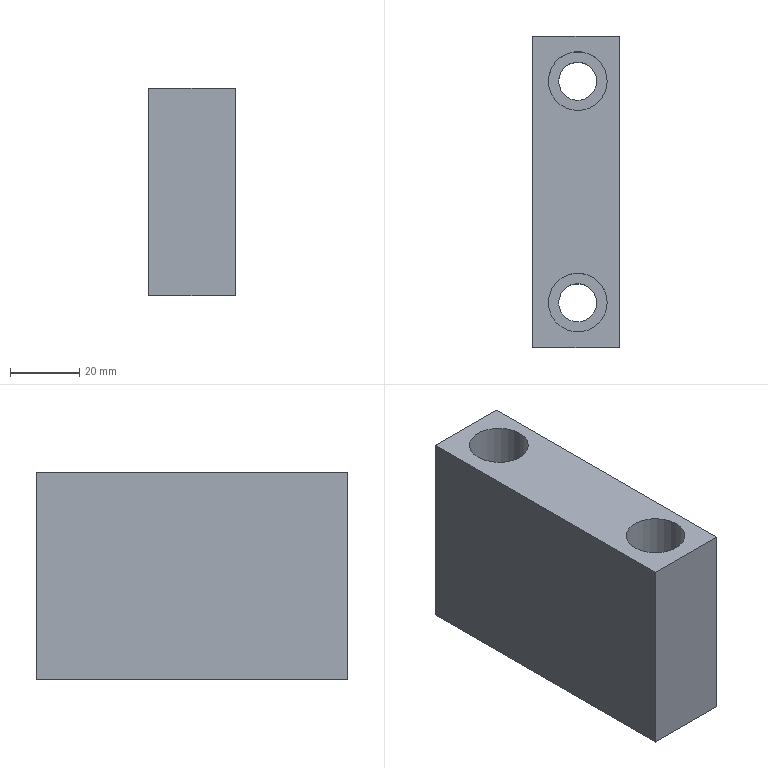Part | STEP file | PN_0005_id1498_x_t | 1 solid | 12 faces | box 25 x 90 x 60 mm | volume 115679 mm3 | plane 8 | cylinder 4 | commonest cylinder face diameters 11 x2 17 x2
STEP:
#1=CARTESIAN_POINT('',(-216.5,194.,155.));
#2=VERTEX_POINT('',#1);
#3=CARTESIAN_POINT('',(-222.,194.,155.));
#4=DIRECTION('',(0.,0.,-1.));
#5=DIRECTION('',(1.,0.,0.));
#6=AXIS2_PLACEMENT_3D('',#3,#4,#5);
#7=CIRCLE('',#6,5.5);
#8=EDGE_CURVE('',#2,#2,#7,.T.);
#9=ORIENTED_EDGE('',*,*,#8,.F.);
#10=EDGE_LOOP('',(#9));
#11=FACE_BOUND('',#10,.T.);
#12=CARTESIAN_POINT('',(-216.5,130.,155.));
#13=VERTEX_POINT('',#12);
#14=CARTESIAN_POINT('',(-222.,130.,155.));
#15=DIRECTION('',(0.,0.,1.));
#16=DIRECTION('',(1.,0.,0.));
#17=AXIS2_PLACEMENT_3D('',#14,#15,#16);
#18=CIRCLE('',#17,5.5);
#19=EDGE_CURVE('',#13,#13,#18,.T.);
#20=ORIENTED_EDGE('',*,*,#19,.T.);
#21=EDGE_LOOP('',(#20));
#22=FACE_BOUND('',#21,.T.);
#23=CARTESIAN_POINT('',(-210.,207.,155.));
#24=VERTEX_POINT('',#23);
#25=CARTESIAN_POINT('',(-235.,207.,155.));
#26=VERTEX_POINT('',#25);
#27=CARTESIAN_POINT('',(-190.,207.,155.));
#28=DIRECTION('',(-1.,0.,0.));
#29=VECTOR('',#28,1.);
#30=LINE('',#27,#29);
#31=EDGE_CURVE('',#24,#26,#30,.T.);
#32=ORIENTED_EDGE('',*,*,#31,.F.);
#33=CARTESIAN_POINT('',(-210.,117.,155.));
#34=VERTEX_POINT('',#33);
#35=CARTESIAN_POINT('',(-210.,-7.4,155.));
#36=DIRECTION('',(0.,-1.,0.));
#37=VECTOR('',#36,1.);
#38=LINE('',#35,#37);
#39=EDGE_CURVE('',#24,#34,#38,.T.);
#40=ORIENTED_EDGE('',*,*,#39,.T.);
#41=CARTESIAN_POINT('',(-235.,117.,155.));
#42=VERTEX_POINT('',#41);
#43=CARTESIAN_POINT('',(-190.,117.,155.));
#44=DIRECTION('',(1.,0.,0.));
#45=VECTOR('',#44,1.);
#46=LINE('',#43,#45);
#47=EDGE_CURVE('',#42,#34,#46,.T.);
#48=ORIENTED_EDGE('',*,*,#47,.F.);
#49=CARTESIAN_POINT('',(-235.,94.6,155.));
#50=DIRECTION('',(0.,-1.,0.));
#51=VECTOR('',#50,1.);
#52=LINE('',#49,#51);
#53=EDGE_CURVE('',#26,#42,#52,.T.);
#54=ORIENTED_EDGE('',*,*,#53,.F.);
#55=EDGE_LOOP('',(#32,#40,#48,#54));
#56=FACE_BOUND('',#55,.T.);
#57=CARTESIAN_POINT('',(223.5,101.,155.));
#58=DIRECTION('',(0.,0.,-1.));
#59=DIRECTION('',(1.,0.,0.));
#60=AXIS2_PLACEMENT_3D('',#57,#58,#59);
#61=PLANE('',#60);
#62=ADVANCED_FACE('',(#11,#22,#56),#61,.T.);
#63=CARTESIAN_POINT('',(-210.,117.,215.));
#64=VERTEX_POINT('',#63);
#65=CARTESIAN_POINT('',(-210.,117.,155.));
#66=DIRECTION('',(0.,0.,-1.));
#67=VECTOR('',#66,1.);
#68=LINE('',#65,#67);
#69=EDGE_CURVE('',#64,#34,#68,.T.);
#70=ORIENTED_EDGE('',*,*,#69,.F.);
#71=CARTESIAN_POINT('',(-235.,117.,215.));
#72=VERTEX_POINT('',#71);
#73=CARTESIAN_POINT('',(-190.,117.,215.));
#74=DIRECTION('',(-1.,0.,0.));
#75=VECTOR('',#74,1.);
#76=LINE('',#73,#75);
#77=EDGE_CURVE('',#64,#72,#76,.T.);
#78=ORIENTED_EDGE('',*,*,#77,.T.);
#79=CARTESIAN_POINT('',(-235.,117.,155.));
#80=DIRECTION('',(0.,0.,-1.));
#81=VECTOR('',#80,1.);
#82=LINE('',#79,#81);
#83=EDGE_CURVE('',#72,#42,#82,.T.);
#84=ORIENTED_EDGE('',*,*,#83,.T.);
#85=ORIENTED_EDGE('',*,*,#47,.T.);
#86=EDGE_LOOP('',(#70,#78,#84,#85));
#87=FACE_OUTER_BOUND('',#86,.T.);
#88=CARTESIAN_POINT('',(-190.,117.,155.));
#89=DIRECTION('',(0.,-1.,0.));
#90=DIRECTION('',(0.,0.,-1.));
#91=AXIS2_PLACEMENT_3D('',#88,#89,#90);
#92=PLANE('',#91);
#93=ADVANCED_FACE('',(#87),#92,.T.);
#94=CARTESIAN_POINT('',(-210.,207.,215.));
#95=VERTEX_POINT('',#94);
#96=CARTESIAN_POINT('',(-210.,207.,155.));
#97=DIRECTION('',(0.,0.,1.));
#98=VECTOR('',#97,1.);
#99=LINE('',#96,#98);
#100=EDGE_CURVE('',#24,#95,#99,.T.);
#101=ORIENTED_EDGE('',*,*,#100,.F.);
#102=ORIENTED_EDGE('',*,*,#31,.T.);
#103=CARTESIAN_POINT('',(-235.,207.,215.));
#104=VERTEX_POINT('',#103);
#105=CARTESIAN_POINT('',(-235.,207.,138.004));
#106=DIRECTION('',(0.,0.,-1.));
#107=VECTOR('',#106,1.);
#108=LINE('',#105,#107);
#109=EDGE_CURVE('',#104,#26,#108,.T.);
#110=ORIENTED_EDGE('',*,*,#109,.F.);
#111=CARTESIAN_POINT('',(-190.,207.,215.));
#112=DIRECTION('',(1.,0.,0.));
#113=VECTOR('',#112,1.);
#114=LINE('',#111,#113);
#115=EDGE_CURVE('',#104,#95,#114,.T.);
#116=ORIENTED_EDGE('',*,*,#115,.T.);
#117=EDGE_LOOP('',(#101,#102,#110,#116));
#118=FACE_OUTER_BOUND('',#117,.T.);
#119=CARTESIAN_POINT('',(-190.,207.,155.));
#120=DIRECTION('',(0.,1.,0.));
#121=DIRECTION('',(0.,0.,1.));
#122=AXIS2_PLACEMENT_3D('',#119,#120,#121);
#123=PLANE('',#122);
#124=ADVANCED_FACE('',(#118),#123,.T.);
#125=CARTESIAN_POINT('',(-230.5,194.,215.));
#126=VERTEX_POINT('',#125);
#127=CARTESIAN_POINT('',(-222.,194.,215.));
#128=DIRECTION('',(0.,0.,1.));
#129=DIRECTION('',(-1.,0.,0.));
#130=AXIS2_PLACEMENT_3D('',#127,#128,#129);
#131=CIRCLE('',#130,8.5);
#132=EDGE_CURVE('',#126,#126,#131,.T.);
#133=ORIENTED_EDGE('',*,*,#132,.F.);
#134=EDGE_LOOP('',(#133));
#135=FACE_BOUND('',#134,.T.);
#136=CARTESIAN_POINT('',(-230.5,130.,215.));
#137=VERTEX_POINT('',#136);
#138=CARTESIAN_POINT('',(-222.,130.,215.));
#139=DIRECTION('',(0.,0.,-1.));
#140=DIRECTION('',(-1.,0.,0.));
#141=AXIS2_PLACEMENT_3D('',#138,#139,#140);
#142=CIRCLE('',#141,8.5);
#143=EDGE_CURVE('',#137,#137,#142,.T.);
#144=ORIENTED_EDGE('',*,*,#143,.T.);
#145=EDGE_LOOP('',(#144));
#146=FACE_BOUND('',#145,.T.);
#147=CARTESIAN_POINT('',(-210.,-7.4,215.));
#148=DIRECTION('',(0.,-1.,0.));
#149=VECTOR('',#148,1.);
#150=LINE('',#147,#149);
#151=EDGE_CURVE('',#95,#64,#150,.T.);
#152=ORIENTED_EDGE('',*,*,#151,.F.);
#153=ORIENTED_EDGE('',*,*,#115,.F.);
#154=CARTESIAN_POINT('',(-235.,94.6,215.));
#155=DIRECTION('',(0.,1.,0.));
#156=VECTOR('',#155,1.);
#157=LINE('',#154,#156);
#158=EDGE_CURVE('',#72,#104,#157,.T.);
#159=ORIENTED_EDGE('',*,*,#158,.F.);
#160=ORIENTED_EDGE('',*,*,#77,.F.);
#161=EDGE_LOOP('',(#152,#153,#159,#160));
#162=FACE_BOUND('',#161,.T.);
#163=CARTESIAN_POINT('',(268.5,101.,215.));
#164=DIRECTION('',(0.,0.,-1.));
#165=DIRECTION('',(1.,0.,0.));
#166=AXIS2_PLACEMENT_3D('',#163,#164,#165);
#167=PLANE('',#166);
#168=ADVANCED_FACE('',(#135,#146,#162),#167,.F.);
#169=ORIENTED_EDGE('',*,*,#158,.T.);
#170=ORIENTED_EDGE('',*,*,#109,.T.);
#171=ORIENTED_EDGE('',*,*,#53,.T.);
#172=ORIENTED_EDGE('',*,*,#83,.F.);
#173=EDGE_LOOP('',(#169,#170,#171,#172));
#174=FACE_OUTER_BOUND('',#173,.T.);
#175=CARTESIAN_POINT('',(-235.,94.6,138.004));
#176=DIRECTION('',(-1.,0.,0.));
#177=DIRECTION('',(0.,0.,-1.));
#178=AXIS2_PLACEMENT_3D('',#175,#176,#177);
#179=PLANE('',#178);
#180=ADVANCED_FACE('',(#174),#179,.T.);
#181=ORIENTED_EDGE('',*,*,#69,.T.);
#182=ORIENTED_EDGE('',*,*,#39,.F.);
#183=ORIENTED_EDGE('',*,*,#100,.T.);
#184=ORIENTED_EDGE('',*,*,#151,.T.);
#185=EDGE_LOOP('',(#181,#182,#183,#184));
#186=FACE_OUTER_BOUND('',#185,.T.);
#187=CARTESIAN_POINT('',(-210.,-7.4,155.));
#188=DIRECTION('',(1.,0.,0.));
#189=DIRECTION('',(0.,-1.,0.));
#190=AXIS2_PLACEMENT_3D('',#187,#188,#189);
#191=PLANE('',#190);
#192=ADVANCED_FACE('',(#186),#191,.T.);
#193=CARTESIAN_POINT('',(-227.5,130.,185.));
#194=VERTEX_POINT('',#193);
#195=CARTESIAN_POINT('',(-222.,130.,185.));
#196=DIRECTION('',(0.,0.,-1.));
#197=DIRECTION('',(-1.,0.,0.));
#198=AXIS2_PLACEMENT_3D('',#195,#196,#197);
#199=CIRCLE('',#198,5.5);
#200=EDGE_CURVE('',#194,#194,#199,.T.);
#201=ORIENTED_EDGE('',*,*,#200,.F.);
#202=EDGE_LOOP('',(#201));
#203=FACE_BOUND('',#202,.T.);
#204=ORIENTED_EDGE('',*,*,#19,.F.);
#205=EDGE_LOOP('',(#204));
#206=FACE_BOUND('',#205,.T.);
#207=CARTESIAN_POINT('',(-222.,130.,155.));
#208=DIRECTION('',(0.,0.,1.));
#209=DIRECTION('',(1.,0.,0.));
#210=AXIS2_PLACEMENT_3D('',#207,#208,#209);
#211=CYLINDRICAL_SURFACE('',#210,5.5);
#212=ADVANCED_FACE('',(#203,#206),#211,.F.);
#213=ORIENTED_EDGE('',*,*,#200,.T.);
#214=EDGE_LOOP('',(#213));
#215=FACE_BOUND('',#214,.T.);
#216=CARTESIAN_POINT('',(-213.5,130.,185.));
#217=VERTEX_POINT('',#216);
#218=CARTESIAN_POINT('',(-222.,130.,185.));
#219=DIRECTION('',(0.,0.,-1.));
#220=DIRECTION('',(1.,0.,0.));
#221=AXIS2_PLACEMENT_3D('',#218,#219,#220);
#222=CIRCLE('',#221,8.5);
#223=EDGE_CURVE('',#217,#217,#222,.T.);
#224=ORIENTED_EDGE('',*,*,#223,.F.);
#225=EDGE_LOOP('',(#224));
#226=FACE_BOUND('',#225,.T.);
#227=CARTESIAN_POINT('',(-222.,130.,185.));
#228=DIRECTION('',(0.,0.,-1.));
#229=DIRECTION('',(-1.,0.,0.));
#230=AXIS2_PLACEMENT_3D('',#227,#228,#229);
#231=PLANE('',#230);
#232=ADVANCED_FACE('',(#215,#226),#231,.F.);
#233=ORIENTED_EDGE('',*,*,#143,.F.);
#234=EDGE_LOOP('',(#233));
#235=FACE_BOUND('',#234,.T.);
#236=ORIENTED_EDGE('',*,*,#223,.T.);
#237=EDGE_LOOP('',(#236));
#238=FACE_BOUND('',#237,.T.);
#239=CARTESIAN_POINT('',(-222.,130.,185.));
#240=DIRECTION('',(0.,0.,1.));
#241=DIRECTION('',(1.,0.,0.));
#242=AXIS2_PLACEMENT_3D('',#239,#240,#241);
#243=CYLINDRICAL_SURFACE('',#242,8.5);
#244=ADVANCED_FACE('',(#235,#238),#243,.F.);
#245=CARTESIAN_POINT('',(-227.5,194.,185.));
#246=VERTEX_POINT('',#245);
#247=CARTESIAN_POINT('',(-222.,194.,185.));
#248=DIRECTION('',(0.,0.,1.));
#249=DIRECTION('',(-1.,0.,0.));
#250=AXIS2_PLACEMENT_3D('',#247,#248,#249);
#251=CIRCLE('',#250,5.5);
#252=EDGE_CURVE('',#246,#246,#251,.T.);
#253=ORIENTED_EDGE('',*,*,#252,.T.);
#254=EDGE_LOOP('',(#253));
#255=FACE_BOUND('',#254,.T.);
#256=ORIENTED_EDGE('',*,*,#8,.T.);
#257=EDGE_LOOP('',(#256));
#258=FACE_BOUND('',#257,.T.);
#259=CARTESIAN_POINT('',(-222.,194.,155.));
#260=DIRECTION('',(0.,0.,1.));
#261=DIRECTION('',(1.,0.,0.));
#262=AXIS2_PLACEMENT_3D('',#259,#260,#261);
#263=CYLINDRICAL_SURFACE('',#262,5.5);
#264=ADVANCED_FACE('',(#255,#258),#263,.F.);
#265=ORIENTED_EDGE('',*,*,#252,.F.);
#266=EDGE_LOOP('',(#265));
#267=FACE_BOUND('',#266,.T.);
#268=CARTESIAN_POINT('',(-213.5,194.,185.));
#269=VERTEX_POINT('',#268);
#270=CARTESIAN_POINT('',(-222.,194.,185.));
#271=DIRECTION('',(0.,0.,1.));
#272=DIRECTION('',(1.,0.,0.));
#273=AXIS2_PLACEMENT_3D('',#270,#271,#272);
#274=CIRCLE('',#273,8.5);
#275=EDGE_CURVE('',#269,#269,#274,.T.);
#276=ORIENTED_EDGE('',*,*,#275,.T.);
#277=EDGE_LOOP('',(#276));
#278=FACE_BOUND('',#277,.T.);
#279=CARTESIAN_POINT('',(-222.,194.,185.));
#280=DIRECTION('',(0.,0.,-1.));
#281=DIRECTION('',(-1.,0.,0.));
#282=AXIS2_PLACEMENT_3D('',#279,#280,#281);
#283=PLANE('',#282);
#284=ADVANCED_FACE('',(#267,#278),#283,.F.);
#285=ORIENTED_EDGE('',*,*,#132,.T.);
#286=EDGE_LOOP('',(#285));
#287=FACE_BOUND('',#286,.T.);
#288=ORIENTED_EDGE('',*,*,#275,.F.);
#289=EDGE_LOOP('',(#288));
#290=FACE_BOUND('',#289,.T.);
#291=CARTESIAN_POINT('',(-222.,194.,185.));
#292=DIRECTION('',(0.,0.,1.));
#293=DIRECTION('',(1.,0.,0.));
#294=AXIS2_PLACEMENT_3D('',#291,#292,#293);
#295=CYLINDRICAL_SURFACE('',#294,8.5);
#296=ADVANCED_FACE('',(#287,#290),#295,.F.);
#297=CLOSED_SHELL('',(#62,#93,#124,#168,#180,#192,#212,#232,#244,#264,#284,#296));
#298=MANIFOLD_SOLID_BREP('',#297);
#299=(LENGTH_UNIT()NAMED_UNIT(*)SI_UNIT(.MILLI.,.METRE.));
#300=UNCERTAINTY_MEASURE_WITH_UNIT(LENGTH_MEASURE(0.00002),#299,'','');
#301=(NAMED_UNIT(*)PLANE_ANGLE_UNIT()SI_UNIT($,.RADIAN.));
#302=PLANE_ANGLE_MEASURE_WITH_UNIT(PLANE_ANGLE_MEASURE(0.01745),#301);
#303=DIMENSIONAL_EXPONENTS(0.,0.,0.,0.,0.,0.,0.);
#304=(CONVERSION_BASED_UNIT('DEGREE',#302)NAMED_UNIT(#303)PLANE_ANGLE_UNIT());
#305=(NAMED_UNIT(*)SI_UNIT($,.STERADIAN.)SOLID_ANGLE_UNIT());
#306=(GEOMETRIC_REPRESENTATION_CONTEXT(3)GLOBAL_UNCERTAINTY_ASSIGNED_CONTEXT((#300))GLOBAL_UNIT_ASSIGNED_CONTEXT((#299,#304,#305))REPRESENTATION_CONTEXT('',''));
#307=ADVANCED_BREP_SHAPE_REPRESENTATION('',(#298),#306);